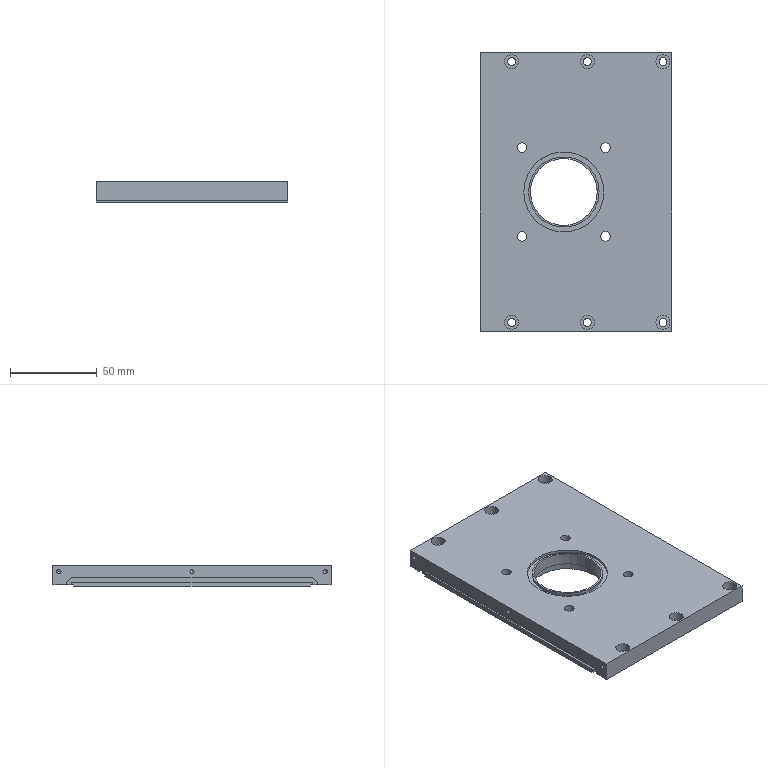NC program | NX | posted with a generic post | part box 110 x 160 x 12 mm
Lines 31 to 887 of 4419:
(ZLEVEL_PROFILE_COPY , TOOL : D3)
N54 T17 M6
N56 G54
N58 G17 G0 G90 X-46.066 Y1.694 B0. C0. S6260 M3
N60 G43 Z30. H17
N62 Z1.
N64 G94 G1 X-46.26 Y1.5 Z0.986 F1100.
N66 X-46.397 Y1.154 Z0.966
N68 X-46.384 Y0.783 Z0.947
N70 X-46.223 Y0.448 Z0.927
N72 X-46.03 Y0.261 Z0.913
N74 X-45.842 Y0.157 Z0.902
N76 X-45.635 Y0.1 Z0.891
N78 X-44.365 Z0.824
N80 X-44.064 Y0.201 Z0.807
N82 X-43.816 Y0.4 Z0.791
N84 X-43.651 Y0.672 Z0.774
N86 X-43.592 Y0.934 Z0.76
N88 X-43.631 Y1.27 Z0.742
N90 X-43.79 Y1.569 Z0.725
N92 X-44.046 Y1.789 Z0.707
N94 X-44.365 Y1.9 Z0.689
N96 X-45.635 Z0.623
N98 X-45.753 Y1.874 Z0.616
N100 X-45.997 Y1.762 Z0.602
N102 X-46.26 Y1.5 Z0.583
N104 X-46.397 Y1.154 Z0.563
N106 X-46.384 Y0.783 Z0.544
N108 X-46.223 Y0.448 Z0.524
N110 X-46.03 Y0.261 Z0.51
N112 X-45.842 Y0.157 Z0.499
N114 X-45.635 Y0.1 Z0.488
N116 X-44.365 Z0.421
N118 X-44.064 Y0.201 Z0.404
N120 X-43.816 Y0.4 Z0.388
N122 X-43.651 Y0.672 Z0.371
N124 X-43.592 Y0.934 Z0.357
N126 X-43.631 Y1.27 Z0.339
N128 X-43.79 Y1.569 Z0.322
N130 X-44.046 Y1.789 Z0.304
N132 X-44.365 Y1.9 Z0.286
N134 X-45.635 Z0.22
N136 X-45.753 Y1.874 Z0.213
N138 X-45.997 Y1.762 Z0.199
N140 X-46.26 Y1.5 Z0.18
N142 X-46.397 Y1.154 Z0.16
N144 X-46.384 Y0.783 Z0.141
N146 X-46.223 Y0.448 Z0.121
N148 X-46.03 Y0.261 Z0.107
N150 X-45.842 Y0.157 Z0.096
N152 X-45.635 Y0.1 Z0.085
N154 X-44.365 Z0.018
N156 X-44.064 Y0.201 Z0.002
N158 X-43.816 Y0.4 Z-0.015
N160 X-43.651 Y0.672 Z-0.032
N162 X-43.592 Y0.934 Z-0.046
N164 X-43.631 Y1.27 Z-0.064
N166 X-43.79 Y1.569 Z-0.081
N168 X-44.046 Y1.789 Z-0.099
N170 X-44.365 Y1.9 Z-0.117
N172 X-45. Z-0.15
N174 X-45.5
N176 G3 X-46.4 Y1. R0.9
N178 X-45.5 Y0.1 R0.9
N180 G1 X-44.5
N182 G3 X-43.6 Y1. R0.9
N184 X-44.5 Y1.9 R0.9
N186 G1 X-45.
N188 X-45.374 Z-0.16
N190 X-45.499 Y1.894 Z-0.163
N192 X-45.676 Y1.874 Z-0.168
N194 X-45.743 Y1.857 Z-0.17
N196 X-45.891 Y1.801 Z-0.174
N198 X-45.969 Y1.759 Z-0.176
N200 X-46.049 Y1.703 Z-0.179
N202 X-46.087 Y1.673 Z-0.18
N204 X-46.111 Y1.649 Z-0.181
N206 X-46.159 Y1.601 Z-0.183
N208 X-46.247 Y1.487 Z-0.186
N210 X-46.297 Y1.397 Z-0.189
N212 X-46.354 Y1.254 Z-0.193
N214 X-46.379 Y1.164 Z-0.196
N216 X-46.392 Y1.035 Z-0.199
N218 X-46.387 Y0.918 Z-0.202
N220 X-46.36 Y0.769 Z-0.206
N222 X-46.332 Y0.677 Z-0.209
N224 X-46.295 Y0.596 Z-0.211
N226 X-46.275 Y0.555 Z-0.212
N228 X-46.254 Y0.524 Z-0.213
N230 X-46.211 Y0.463 Z-0.215
N232 X-46.11 Y0.351 Z-0.219
N234 X-46.037 Y0.289 Z-0.222
N236 X-45.908 Y0.207 Z-0.226
N238 X-45.822 Y0.167 Z-0.228
N240 X-45.717 Y0.136 Z-0.231
N242 X-45.581 Y0.113 Z-0.235
N244 X-45.457 Y0.102 Z-0.238
N246 X-45.333 Y0.1 Z-0.241
N248 X-44.584 Z-0.261
N250 X-44.4 Y0.114 Z-0.266
N252 X-44.336 Y0.121 Z-0.267
N254 X-44.251 Y0.144 Z-0.27
N256 X-44.208 Y0.156 Z-0.271
N258 X-44.172 Y0.17 Z-0.272
N260 X-44.103 Y0.202 Z-0.274
N262 X-43.967 Y0.286 Z-0.278
N264 X-43.899 Y0.341 Z-0.28
N266 X-43.8 Y0.447 Z-0.284
N268 X-43.742 Y0.53 Z-0.287
N270 X-43.68 Y0.65 Z-0.291
N272 X-43.643 Y0.756 Z-0.293
N274 X-43.617 Y0.877 Z-0.297
N276 X-43.6 Y1. Z-0.3
N278 G3 X-44.5 Y1.9 R0.9
N280 G1 X-45.
N282 X-45.374 Z-0.31
N284 X-45.499 Y1.894 Z-0.313
N286 X-45.677 Y1.875 Z-0.318
N288 X-45.743 Y1.857 Z-0.32
N290 X-45.896 Y1.798 Z-0.324
N292 X-45.969 Y1.759 Z-0.326
N294 X-46.05 Y1.703 Z-0.329
N296 X-46.088 Y1.672 Z-0.33
N298 X-46.111 Y1.649 Z-0.331
N300 X-46.159 Y1.601 Z-0.333
N302 X-46.247 Y1.487 Z-0.336
N304 X-46.297 Y1.397 Z-0.339
N306 X-46.354 Y1.254 Z-0.343
N308 X-46.379 Y1.164 Z-0.346
N310 X-46.392 Y1.035 Z-0.349
N312 X-46.387 Y0.918 Z-0.352
N314 X-46.36 Y0.769 Z-0.356
N316 X-46.332 Y0.677 Z-0.359
N318 X-46.295 Y0.596 Z-0.361
N320 X-46.275 Y0.555 Z-0.362
N322 X-46.254 Y0.524 Z-0.363
N324 X-46.211 Y0.463 Z-0.365
N326 X-46.11 Y0.351 Z-0.369
N328 X-46.037 Y0.289 Z-0.372
N330 X-45.908 Y0.207 Z-0.376
N332 X-45.822 Y0.167 Z-0.378
N334 X-45.717 Y0.136 Z-0.381
N336 X-45.581 Y0.113 Z-0.385
N338 X-45.457 Y0.102 Z-0.388
N340 X-45.333 Y0.1 Z-0.391
N342 X-44.584 Z-0.411
N344 X-44.4 Y0.114 Z-0.416
N346 X-44.336 Y0.121 Z-0.417
N348 X-44.251 Y0.144 Z-0.42
N350 X-44.208 Y0.156 Z-0.421
N352 X-44.172 Y0.17 Z-0.422
N354 X-44.103 Y0.202 Z-0.424
N356 X-43.967 Y0.286 Z-0.428
N358 X-43.899 Y0.341 Z-0.43
N360 X-43.8 Y0.447 Z-0.434
N362 X-43.742 Y0.53 Z-0.437
N364 X-43.68 Y0.65 Z-0.441
N366 X-43.643 Y0.756 Z-0.443
N368 X-43.617 Y0.877 Z-0.447
N370 X-43.6 Y1. Z-0.45
N372 G3 X-44.5 Y1.9 R0.9
N374 G1 X-45.
N376 X-45.374 Z-0.46
N378 X-45.499 Y1.894 Z-0.463
N380 X-45.677 Y1.875 Z-0.468
N382 X-45.743 Y1.857 Z-0.47
N384 X-45.896 Y1.798 Z-0.474
N386 X-45.969 Y1.759 Z-0.476
N388 X-46.05 Y1.703 Z-0.479
N390 X-46.088 Y1.672 Z-0.48
N392 X-46.111 Y1.649 Z-0.481
N394 X-46.159 Y1.601 Z-0.483
N396 X-46.247 Y1.487 Z-0.486
N398 X-46.297 Y1.397 Z-0.489
N400 X-46.354 Y1.254 Z-0.493
N402 X-46.379 Y1.164 Z-0.496
N404 X-46.391 Y1.035 Z-0.499
N406 X-46.387 Y0.918 Z-0.502
N408 X-46.36 Y0.769 Z-0.506
N410 X-46.332 Y0.677 Z-0.509
N412 X-46.295 Y0.596 Z-0.511
N414 X-46.275 Y0.555 Z-0.512
N416 X-46.254 Y0.524 Z-0.513
N418 X-46.211 Y0.463 Z-0.515
N420 X-46.11 Y0.351 Z-0.519
N422 X-46.036 Y0.289 Z-0.522
N424 X-45.908 Y0.207 Z-0.526
N426 X-45.822 Y0.167 Z-0.528
N428 X-45.717 Y0.136 Z-0.531
N430 X-45.581 Y0.113 Z-0.535
N432 X-45.457 Y0.102 Z-0.538
N434 X-45.333 Y0.1 Z-0.541
N436 X-44.584 Z-0.561
N438 X-44.4 Y0.114 Z-0.566
N440 X-44.336 Y0.121 Z-0.567
N442 X-44.251 Y0.144 Z-0.57
N444 X-44.208 Y0.156 Z-0.571
N446 X-44.172 Y0.17 Z-0.572
N448 X-44.103 Y0.202 Z-0.574
N450 X-43.967 Y0.286 Z-0.578
N452 X-43.899 Y0.341 Z-0.58
N454 X-43.8 Y0.447 Z-0.584
N456 X-43.742 Y0.53 Z-0.587
N458 X-43.681 Y0.65 Z-0.59
N460 X-43.643 Y0.756 Z-0.593
N462 X-43.617 Y0.877 Z-0.597
N464 X-43.6 Y1. Z-0.6
N466 G3 X-44.5 Y1.9 R0.9
N468 G1 X-45.
N470 X-45.374 Z-0.61
N472 X-45.499 Y1.894 Z-0.613
N474 X-45.677 Y1.875 Z-0.618
N476 X-45.743 Y1.857 Z-0.62
N478 X-45.896 Y1.798 Z-0.624
N480 X-45.969 Y1.758 Z-0.626
N482 X-46.049 Y1.703 Z-0.629
N484 X-46.088 Y1.672 Z-0.63
N486 X-46.111 Y1.649 Z-0.631
N488 X-46.159 Y1.601 Z-0.633
N490 X-46.246 Y1.487 Z-0.636
N492 X-46.297 Y1.397 Z-0.639
N494 X-46.354 Y1.254 Z-0.643
N496 X-46.379 Y1.164 Z-0.646
N498 X-46.391 Y1.035 Z-0.649
N500 X-46.387 Y0.918 Z-0.652
N502 X-46.36 Y0.769 Z-0.656
N504 X-46.332 Y0.677 Z-0.659
N506 X-46.295 Y0.596 Z-0.661
N508 X-46.275 Y0.556 Z-0.662
N510 X-46.254 Y0.524 Z-0.663
N512 X-46.211 Y0.463 Z-0.665
N514 X-46.11 Y0.351 Z-0.669
N516 X-46.036 Y0.289 Z-0.672
N518 X-45.908 Y0.208 Z-0.676
N520 X-45.822 Y0.167 Z-0.678
N522 X-45.717 Y0.136 Z-0.681
N524 X-45.581 Y0.113 Z-0.685
N526 X-45.457 Y0.102 Z-0.688
N528 X-45.333 Y0.1 Z-0.691
N530 X-44.584 Z-0.711
N532 X-44.4 Y0.114 Z-0.716
N534 X-44.336 Y0.121 Z-0.717
N536 X-44.251 Y0.144 Z-0.72
N538 X-44.208 Y0.156 Z-0.721
N540 X-44.172 Y0.17 Z-0.722
N542 X-44.103 Y0.202 Z-0.724
N544 X-43.967 Y0.286 Z-0.728
N546 X-43.9 Y0.341 Z-0.73
N548 X-43.8 Y0.447 Z-0.734
N550 X-43.742 Y0.53 Z-0.737
N552 X-43.681 Y0.65 Z-0.74
N554 X-43.643 Y0.756 Z-0.743
N556 X-43.617 Y0.877 Z-0.747
N558 X-43.6 Y1. Z-0.75
N560 G3 X-44.5 Y1.9 R0.9
N562 G1 X-45.
N564 X-45.374 Z-0.76
N566 X-45.499 Y1.894 Z-0.763
N568 X-45.677 Y1.875 Z-0.768
N570 X-45.743 Y1.857 Z-0.77
N572 X-45.896 Y1.798 Z-0.774
N574 X-45.969 Y1.758 Z-0.776
N576 X-46.049 Y1.703 Z-0.779
N578 X-46.087 Y1.672 Z-0.78
N580 X-46.111 Y1.649 Z-0.781
N582 X-46.159 Y1.601 Z-0.783
N584 X-46.246 Y1.487 Z-0.786
N586 X-46.297 Y1.397 Z-0.789
N588 X-46.354 Y1.254 Z-0.793
N590 X-46.379 Y1.164 Z-0.796
N592 X-46.391 Y1.035 Z-0.799
N594 X-46.387 Y0.918 Z-0.802
N596 X-46.36 Y0.769 Z-0.806
N598 X-46.332 Y0.677 Z-0.809
N600 X-46.295 Y0.596 Z-0.811
N602 X-46.275 Y0.556 Z-0.812
N604 X-46.254 Y0.525 Z-0.813
N606 X-46.211 Y0.463 Z-0.815
N608 X-46.11 Y0.351 Z-0.819
N610 X-46.036 Y0.289 Z-0.822
N612 X-45.908 Y0.208 Z-0.826
N614 X-45.822 Y0.167 Z-0.828
N616 X-45.717 Y0.136 Z-0.831
N618 X-45.581 Y0.113 Z-0.835
N620 X-45.457 Y0.102 Z-0.838
N622 X-45.333 Y0.1 Z-0.841
N624 X-44.584 Z-0.861
N626 X-44.4 Y0.114 Z-0.866
N628 X-44.336 Y0.121 Z-0.867
N630 X-44.251 Y0.144 Z-0.87
N632 X-44.208 Y0.156 Z-0.871
N634 X-44.172 Y0.17 Z-0.872
N636 X-44.103 Y0.202 Z-0.874
N638 X-43.968 Y0.286 Z-0.878
N640 X-43.9 Y0.341 Z-0.88
N642 X-43.8 Y0.447 Z-0.884
N644 X-43.742 Y0.53 Z-0.887
N646 X-43.681 Y0.65 Z-0.89
N648 X-43.643 Y0.756 Z-0.893
N650 X-43.617 Y0.877 Z-0.897
N652 X-43.6 Y1. Z-0.9
N654 G3 X-44.5 Y1.9 R0.9
N656 G1 X-45.
N658 X-45.374 Z-0.91
N660 X-45.499 Y1.894 Z-0.913
N662 X-45.677 Y1.875 Z-0.918
N664 X-45.743 Y1.857 Z-0.92
N666 X-45.896 Y1.798 Z-0.924
N668 X-45.969 Y1.758 Z-0.926
N670 X-46.049 Y1.703 Z-0.929
N672 X-46.087 Y1.672 Z-0.93
N674 X-46.111 Y1.649 Z-0.931
N676 X-46.159 Y1.601 Z-0.933
N678 X-46.246 Y1.487 Z-0.936
N680 X-46.297 Y1.397 Z-0.939
N682 X-46.354 Y1.254 Z-0.943
N684 X-46.379 Y1.164 Z-0.946
N686 X-46.391 Y1.035 Z-0.949
N688 X-46.387 Y0.918 Z-0.952
N690 X-46.36 Y0.769 Z-0.956
N692 X-46.332 Y0.677 Z-0.959
N694 X-46.295 Y0.596 Z-0.961
N696 X-46.275 Y0.556 Z-0.962
N698 X-46.254 Y0.525 Z-0.963
N700 X-46.211 Y0.463 Z-0.965
N702 X-46.11 Y0.351 Z-0.969
N704 X-46.036 Y0.289 Z-0.972
N706 X-45.908 Y0.208 Z-0.976
N708 X-45.822 Y0.167 Z-0.978
N710 X-45.717 Y0.136 Z-0.981
N712 X-45.581 Y0.113 Z-0.985
N714 X-45.457 Y0.102 Z-0.988
N716 X-45.333 Y0.1 Z-0.991
N718 X-44.584 Z-1.011
N720 X-44.4 Y0.114 Z-1.016
N722 X-44.336 Y0.121 Z-1.017
N724 X-44.208 Y0.156 Z-1.021
N726 X-44.103 Y0.202 Z-1.024
N728 X-43.975 Y0.281 Z-1.028
N730 X-43.9 Y0.341 Z-1.03
N732 X-43.832 Y0.409 Z-1.033
N734 X-43.801 Y0.444 Z-1.034
N736 X-43.781 Y0.473 Z-1.035
N738 X-43.742 Y0.53 Z-1.037
N740 X-43.68 Y0.652 Z-1.041
N742 X-43.643 Y0.756 Z-1.043
N744 X-43.617 Y0.877 Z-1.047
N746 X-43.6 Y1. Z-1.05
N748 G3 X-44.5 Y1.9 R0.9
N750 G1 X-45.
N752 X-45.374 Z-1.06
N754 X-45.499 Y1.894 Z-1.063
N756 X-45.677 Y1.875 Z-1.068
N758 X-45.743 Y1.857 Z-1.07
N760 X-45.896 Y1.798 Z-1.074
N762 X-45.969 Y1.758 Z-1.076
N764 X-46.049 Y1.703 Z-1.079
N766 X-46.087 Y1.672 Z-1.08
N768 X-46.111 Y1.649 Z-1.081
N770 X-46.159 Y1.601 Z-1.083
N772 X-46.246 Y1.487 Z-1.086
N774 X-46.297 Y1.397 Z-1.089
N776 X-46.354 Y1.254 Z-1.093
N778 X-46.378 Y1.164 Z-1.096
N780 X-46.391 Y1.035 Z-1.099
N782 X-46.387 Y0.918 Z-1.102
N784 X-46.36 Y0.769 Z-1.106
N786 X-46.332 Y0.677 Z-1.109
N788 X-46.295 Y0.596 Z-1.111
N790 X-46.275 Y0.556 Z-1.112
N792 X-46.254 Y0.525 Z-1.113
N794 X-46.211 Y0.463 Z-1.115
N796 X-46.111 Y0.351 Z-1.119
N798 X-46.036 Y0.289 Z-1.122
N800 X-45.908 Y0.208 Z-1.126
N802 X-45.822 Y0.167 Z-1.128
N804 X-45.718 Y0.136 Z-1.131
N806 X-45.581 Y0.113 Z-1.135
N808 X-45.457 Y0.102 Z-1.138
N810 X-45.333 Y0.1 Z-1.141
N812 X-44.584 Z-1.161
N814 X-44.4 Y0.114 Z-1.166
N816 X-44.336 Y0.121 Z-1.167
N818 X-44.208 Y0.156 Z-1.171
N820 X-44.103 Y0.202 Z-1.174
N822 X-43.975 Y0.281 Z-1.178
N824 X-43.9 Y0.341 Z-1.18
N826 X-43.832 Y0.408 Z-1.183
N828 X-43.801 Y0.444 Z-1.184
N830 X-43.781 Y0.473 Z-1.185
N832 X-43.742 Y0.53 Z-1.187
N834 X-43.68 Y0.652 Z-1.191
N836 X-43.643 Y0.756 Z-1.193
N838 X-43.617 Y0.877 Z-1.197
N840 X-43.6 Y1. Z-1.2
N842 G3 X-44.5 Y1.9 R0.9
N844 G1 X-45.
N846 X-45.374 Z-1.21
N848 X-45.499 Y1.894 Z-1.213
N850 X-45.677 Y1.875 Z-1.218
N852 X-45.743 Y1.857 Z-1.22
N854 X-45.895 Y1.798 Z-1.224
N856 X-45.969 Y1.758 Z-1.226
N858 X-46.049 Y1.703 Z-1.229
N860 X-46.087 Y1.672 Z-1.23
N862 X-46.111 Y1.649 Z-1.231
N864 X-46.159 Y1.601 Z-1.233
N866 X-46.246 Y1.487 Z-1.236
N868 X-46.297 Y1.397 Z-1.239
N870 X-46.354 Y1.254 Z-1.243
N872 X-46.378 Y1.164 Z-1.246
N874 X-46.391 Y1.035 Z-1.249
N876 X-46.387 Y0.918 Z-1.252
N878 X-46.36 Y0.769 Z-1.256
N880 X-46.332 Y0.677 Z-1.259
N882 X-46.295 Y0.596 Z-1.261
N884 X-46.275 Y0.556 Z-1.262
N886 X-46.254 Y0.525 Z-1.263
N888 X-46.211 Y0.463 Z-1.265
N890 X-46.111 Y0.351 Z-1.269
N892 X-46.036 Y0.289 Z-1.272
N894 X-45.908 Y0.208 Z-1.276
N896 X-45.822 Y0.167 Z-1.278
N898 X-45.718 Y0.136 Z-1.281
N900 X-45.581 Y0.113 Z-1.285
N902 X-45.457 Y0.102 Z-1.288
N904 X-45.333 Y0.1 Z-1.291
N906 X-44.584 Z-1.311
N908 X-44.4 Y0.114 Z-1.316
N910 X-44.336 Y0.121 Z-1.317
N912 X-44.208 Y0.156 Z-1.321
N914 X-44.103 Y0.202 Z-1.324
N916 X-43.975 Y0.281 Z-1.328
N918 X-43.9 Y0.341 Z-1.33
N920 X-43.832 Y0.408 Z-1.333
N922 X-43.801 Y0.444 Z-1.334
N924 X-43.782 Y0.473 Z-1.335
N926 X-43.742 Y0.53 Z-1.337
N928 X-43.68 Y0.652 Z-1.341
N930 X-43.643 Y0.756 Z-1.343
N932 X-43.617 Y0.877 Z-1.347
N934 X-43.6 Y1. Z-1.35
N936 G3 X-44.5 Y1.9 R0.9
N938 G1 X-45.
N940 X-45.374 Z-1.36
N942 X-45.499 Y1.894 Z-1.363
N944 X-45.677 Y1.875 Z-1.368
N946 X-45.743 Y1.857 Z-1.37
N948 X-45.895 Y1.798 Z-1.374
N950 X-45.969 Y1.758 Z-1.376
N952 X-46.049 Y1.703 Z-1.379
N954 X-46.087 Y1.672 Z-1.38
N956 X-46.111 Y1.649 Z-1.381
N958 X-46.159 Y1.601 Z-1.383
N960 X-46.246 Y1.487 Z-1.386
N962 X-46.297 Y1.397 Z-1.389
N964 X-46.354 Y1.254 Z-1.393
N966 X-46.378 Y1.164 Z-1.396
N968 X-46.391 Y1.035 Z-1.399
N970 X-46.387 Y0.918 Z-1.402
N972 X-46.36 Y0.77 Z-1.406
N974 X-46.332 Y0.677 Z-1.409
N976 X-46.295 Y0.596 Z-1.411
N978 X-46.275 Y0.556 Z-1.412
N980 X-46.254 Y0.525 Z-1.413
N982 X-46.211 Y0.463 Z-1.415
N984 X-46.111 Y0.351 Z-1.419
N986 X-46.036 Y0.289 Z-1.422
N988 X-45.908 Y0.208 Z-1.426
N990 X-45.822 Y0.167 Z-1.428
N992 X-45.718 Y0.136 Z-1.431
N994 X-45.581 Y0.113 Z-1.435
N996 X-45.457 Y0.102 Z-1.438
N998 X-45.333 Y0.1 Z-1.441
N1000 X-44.584 Z-1.461
N1002 X-44.4 Y0.114 Z-1.466
N1004 X-44.336 Y0.121 Z-1.467
N1006 X-44.208 Y0.156 Z-1.471
N1008 X-44.103 Y0.202 Z-1.474
N1010 X-43.975 Y0.281 Z-1.478
N1012 X-43.9 Y0.341 Z-1.48
N1014 X-43.833 Y0.408 Z-1.483
N1016 X-43.801 Y0.444 Z-1.484
N1018 X-43.782 Y0.473 Z-1.485
N1020 X-43.742 Y0.53 Z-1.487
N1022 X-43.68 Y0.652 Z-1.491
N1024 X-43.643 Y0.756 Z-1.493
N1026 X-43.617 Y0.877 Z-1.497
N1028 X-43.6 Y1. Z-1.5
N1030 G3 X-44.5 Y1.9 R0.9
N1032 G1 X-45.
N1034 X-45.374 Z-1.51
N1036 X-45.499 Y1.894 Z-1.513
N1038 X-45.677 Y1.875 Z-1.518
N1040 X-45.743 Y1.857 Z-1.52
N1042 X-45.895 Y1.798 Z-1.524
N1044 X-45.969 Y1.758 Z-1.526
N1046 X-46.049 Y1.703 Z-1.529
N1048 X-46.087 Y1.673 Z-1.53
N1050 X-46.111 Y1.649 Z-1.531
N1052 X-46.159 Y1.601 Z-1.533
N1054 X-46.246 Y1.488 Z-1.536
N1056 X-46.297 Y1.397 Z-1.539
N1058 X-46.354 Y1.254 Z-1.543
N1060 X-46.378 Y1.164 Z-1.546
N1062 X-46.391 Y1.035 Z-1.549
N1064 X-46.387 Y0.918 Z-1.552
N1066 X-46.36 Y0.77 Z-1.556
N1068 X-46.332 Y0.677 Z-1.559
N1070 X-46.295 Y0.596 Z-1.561
N1072 X-46.275 Y0.556 Z-1.562
N1074 X-46.254 Y0.525 Z-1.563
N1076 X-46.211 Y0.463 Z-1.565
N1078 X-46.111 Y0.351 Z-1.569
N1080 X-46.036 Y0.289 Z-1.572
N1082 X-45.908 Y0.208 Z-1.576
N1084 X-45.822 Y0.167 Z-1.578
N1086 X-45.718 Y0.136 Z-1.581
N1088 X-45.581 Y0.113 Z-1.585
N1090 X-45.457 Y0.102 Z-1.588
N1092 X-45.333 Y0.1 Z-1.591
N1094 X-44.584 Z-1.611
N1096 X-44.401 Y0.114 Z-1.616
N1098 X-44.336 Y0.121 Z-1.617
N1100 X-44.208 Y0.156 Z-1.621
N1102 X-44.103 Y0.202 Z-1.624
N1104 X-43.975 Y0.281 Z-1.628
N1106 X-43.9 Y0.341 Z-1.63
N1108 X-43.801 Y0.444 Z-1.634
N1110 X-43.742 Y0.53 Z-1.637
N1112 X-43.68 Y0.651 Z-1.641
N1114 X-43.643 Y0.756 Z-1.643
N1116 X-43.616 Y0.877 Z-1.647
N1118 X-43.6 Y1. Z-1.65
N1120 G3 X-44.5 Y1.9 R0.9
N1122 G1 X-45.
N1124 X-45.374 Z-1.66
N1126 X-45.499 Y1.894 Z-1.663
N1128 X-45.677 Y1.875 Z-1.668
N1130 X-45.743 Y1.857 Z-1.67
N1132 X-45.895 Y1.798 Z-1.674
N1134 X-45.969 Y1.758 Z-1.676
N1136 X-46.049 Y1.703 Z-1.679
N1138 X-46.087 Y1.673 Z-1.68
N1140 X-46.111 Y1.649 Z-1.681
N1142 X-46.159 Y1.601 Z-1.683
N1144 X-46.246 Y1.488 Z-1.686
N1146 X-46.297 Y1.397 Z-1.689
N1148 X-46.354 Y1.254 Z-1.693
N1150 X-46.378 Y1.164 Z-1.696
N1152 X-46.391 Y1.035 Z-1.699
N1154 X-46.387 Y0.918 Z-1.702
N1156 X-46.361 Y0.769 Z-1.706
N1158 X-46.332 Y0.677 Z-1.709
N1160 X-46.275 Y0.553 Z-1.712
N1162 X-46.211 Y0.463 Z-1.715
N1164 X-46.109 Y0.35 Z-1.719
N1166 X-46.036 Y0.289 Z-1.722
N1168 X-45.908 Y0.208 Z-1.726
N1170 X-45.822 Y0.167 Z-1.728
N1172 X-45.718 Y0.136 Z-1.731
N1174 X-45.581 Y0.113 Z-1.735
N1176 X-45.457 Y0.102 Z-1.738
N1178 X-45.333 Y0.1 Z-1.741
N1180 X-44.584 Z-1.761
N1182 X-44.401 Y0.114 Z-1.766
N1184 X-44.336 Y0.121 Z-1.767
N1186 X-44.208 Y0.156 Z-1.771
N1188 X-44.103 Y0.202 Z-1.774
N1190 X-43.975 Y0.281 Z-1.778
N1192 X-43.9 Y0.341 Z-1.78
N1194 X-43.802 Y0.444 Z-1.784
N1196 X-43.742 Y0.53 Z-1.787
N1198 X-43.68 Y0.651 Z-1.791
N1200 X-43.643 Y0.756 Z-1.793
N1202 X-43.616 Y0.877 Z-1.797
N1204 X-43.6 Y1. Z-1.8
N1206 G3 X-44.5 Y1.9 R0.9
N1208 G1 X-45.
N1210 X-45.374 Z-1.81
N1212 X-45.499 Y1.894 Z-1.813
N1214 X-45.677 Y1.875 Z-1.818
N1216 X-45.743 Y1.857 Z-1.82
N1218 X-45.895 Y1.798 Z-1.824
N1220 X-45.969 Y1.758 Z-1.826
N1222 X-46.087 Y1.673 Z-1.83
N1224 X-46.159 Y1.601 Z-1.833
N1226 X-46.246 Y1.488 Z-1.836
N1228 X-46.297 Y1.397 Z-1.839
N1230 X-46.354 Y1.254 Z-1.843
N1232 X-46.378 Y1.164 Z-1.846
N1234 X-46.391 Y1.035 Z-1.849
N1236 X-46.387 Y0.918 Z-1.852
N1238 X-46.361 Y0.77 Z-1.856
N1240 X-46.332 Y0.677 Z-1.859
N1242 X-46.275 Y0.553 Z-1.862
N1244 X-46.211 Y0.463 Z-1.865
N1246 X-46.109 Y0.35 Z-1.869
N1248 X-46.036 Y0.289 Z-1.872
N1250 X-45.908 Y0.208 Z-1.876
N1252 X-45.822 Y0.167 Z-1.878
N1254 X-45.718 Y0.137 Z-1.881
N1256 X-45.581 Y0.113 Z-1.885
N1258 X-45.457 Y0.102 Z-1.888
N1260 X-45.333 Y0.1 Z-1.891
N1262 X-44.584 Z-1.911
N1264 X-44.401 Y0.114 Z-1.916
N1266 X-44.336 Y0.121 Z-1.917
N1268 X-44.208 Y0.156 Z-1.921
N1270 X-44.103 Y0.202 Z-1.924
N1272 X-43.975 Y0.281 Z-1.928
N1274 X-43.9 Y0.341 Z-1.93
N1276 X-43.802 Y0.444 Z-1.934
N1278 X-43.742 Y0.53 Z-1.937
N1280 X-43.68 Y0.651 Z-1.941
N1282 X-43.643 Y0.756 Z-1.943
N1284 X-43.616 Y0.877 Z-1.947
N1286 X-43.6 Y1. Z-1.95
N1288 G3 X-44.5 Y1.9 R0.9
N1290 G1 X-45.
N1292 X-45.374 Z-1.96
N1294 X-45.499 Y1.894 Z-1.963
N1296 X-45.677 Y1.875 Z-1.968
N1298 X-45.743 Y1.857 Z-1.97
N1300 X-45.895 Y1.798 Z-1.974
N1302 X-45.969 Y1.758 Z-1.976
N1304 X-46.087 Y1.673 Z-1.98
N1306 X-46.159 Y1.601 Z-1.983
N1308 X-46.246 Y1.488 Z-1.986
N1310 X-46.297 Y1.397 Z-1.989
N1312 X-46.354 Y1.254 Z-1.993
N1314 X-46.378 Y1.164 Z-1.996
N1316 X-46.391 Y1.035 Z-1.999
N1318 X-46.387 Y0.918 Z-2.002
N1320 X-46.361 Y0.77 Z-2.006
N1322 X-46.332 Y0.677 Z-2.009
N1324 X-46.275 Y0.553 Z-2.012
N1326 X-46.211 Y0.463 Z-2.015
N1328 X-46.109 Y0.35 Z-2.019
N1330 X-46.036 Y0.289 Z-2.022
N1332 X-45.908 Y0.208 Z-2.026
N1334 X-45.822 Y0.167 Z-2.028
N1336 X-45.718 Y0.137 Z-2.031
N1338 X-45.581 Y0.113 Z-2.035
N1340 X-45.457 Y0.102 Z-2.038
N1342 X-45.333 Y0.1 Z-2.041
N1344 X-44.584 Z-2.061
N1346 X-44.401 Y0.114 Z-2.066
N1348 X-44.336 Y0.121 Z-2.067
N1350 X-44.208 Y0.156 Z-2.071
N1352 X-44.103 Y0.202 Z-2.074
N1354 X-43.975 Y0.281 Z-2.078
N1356 X-43.9 Y0.341 Z-2.08
N1358 X-43.802 Y0.444 Z-2.084
N1360 X-43.742 Y0.53 Z-2.087
N1362 X-43.68 Y0.651 Z-2.091
N1364 X-43.643 Y0.756 Z-2.093
N1366 X-43.616 Y0.877 Z-2.097
N1368 X-43.6 Y1. Z-2.1
N1370 G3 X-44.5 Y1.9 R0.9
N1372 G1 X-45.
N1374 X-45.374 Z-2.11
N1376 X-45.499 Y1.894 Z-2.113
N1378 X-45.677 Y1.875 Z-2.118
N1380 X-45.743 Y1.857 Z-2.12
N1382 X-45.895 Y1.798 Z-2.124
N1384 X-45.969 Y1.758 Z-2.126
N1386 X-46.087 Y1.673 Z-2.13
N1388 X-46.159 Y1.601 Z-2.133
N1390 X-46.245 Y1.488 Z-2.136
N1392 X-46.297 Y1.397 Z-2.139
N1394 X-46.354 Y1.255 Z-2.143
N1396 X-46.378 Y1.164 Z-2.146
N1398 X-46.391 Y1.035 Z-2.149
N1400 X-46.387 Y0.918 Z-2.152
N1402 X-46.361 Y0.77 Z-2.156
N1404 X-46.332 Y0.677 Z-2.159
N1406 X-46.275 Y0.553 Z-2.162
N1408 X-46.211 Y0.463 Z-2.165
N1410 X-46.109 Y0.35 Z-2.169
N1412 X-46.036 Y0.289 Z-2.172
N1414 X-45.908 Y0.208 Z-2.176
N1416 X-45.822 Y0.167 Z-2.178
N1418 X-45.718 Y0.137 Z-2.181
N1420 X-45.581 Y0.113 Z-2.185
N1422 X-45.457 Y0.102 Z-2.188
N1424 X-45.333 Y0.1 Z-2.191
N1426 X-44.584 Z-2.211
N1428 X-44.401 Y0.115 Z-2.216
N1430 X-44.336 Y0.122 Z-2.217
N1432 X-44.209 Y0.156 Z-2.221
N1434 X-44.104 Y0.203 Z-2.224
N1436 X-43.976 Y0.281 Z-2.228
N1438 X-43.9 Y0.341 Z-2.23
N1440 X-43.802 Y0.444 Z-2.234
N1442 X-43.742 Y0.53 Z-2.237
N1444 X-43.68 Y0.651 Z-2.241
N1446 X-43.643 Y0.756 Z-2.243
N1448 X-43.616 Y0.877 Z-2.247
N1450 X-43.6 Y1. Z-2.25
N1452 G3 X-44.5 Y1.9 R0.9
N1454 G1 X-45.
N1456 X-45.374 Z-2.26
N1458 X-45.499 Y1.894 Z-2.263
N1460 X-45.678 Y1.875 Z-2.268
N1462 X-45.743 Y1.857 Z-2.27
N1464 X-45.895 Y1.798 Z-2.274
N1466 X-45.969 Y1.758 Z-2.276
N1468 X-46.087 Y1.673 Z-2.28
N1470 X-46.159 Y1.601 Z-2.283
N1472 X-46.245 Y1.488 Z-2.286
N1474 X-46.297 Y1.397 Z-2.289
N1476 X-46.353 Y1.255 Z-2.293
N1478 X-46.378 Y1.164 Z-2.296
N1480 X-46.391 Y1.036 Z-2.299
N1482 X-46.387 Y0.918 Z-2.302
N1484 X-46.361 Y0.77 Z-2.306
N1486 X-46.332 Y0.677 Z-2.309
N1488 X-46.275 Y0.554 Z-2.312
N1490 X-46.211 Y0.463 Z-2.315
N1492 X-46.109 Y0.35 Z-2.319
N1494 X-46.036 Y0.289 Z-2.322
N1496 X-45.908 Y0.208 Z-2.326
N1498 X-45.822 Y0.167 Z-2.328
N1500 X-45.718 Y0.137 Z-2.331
N1502 X-45.581 Y0.113 Z-2.335
N1504 X-45.457 Y0.102 Z-2.338
N1506 X-45.333 Y0.1 Z-2.341
N1508 X-44.584 Z-2.361
N1510 X-44.401 Y0.115 Z-2.366
N1512 X-44.336 Y0.122 Z-2.367
N1514 X-44.209 Y0.156 Z-2.371
N1516 X-44.104 Y0.203 Z-2.374
N1518 X-43.976 Y0.281 Z-2.378
N1520 X-43.9 Y0.341 Z-2.38
N1522 X-43.802 Y0.444 Z-2.384
N1524 X-43.742 Y0.53 Z-2.387
N1526 X-43.681 Y0.651 Z-2.391
N1528 X-43.643 Y0.756 Z-2.393
N1530 X-43.616 Y0.877 Z-2.397
N1532 X-43.6 Y1. Z-2.4
N1534 G3 X-44.5 Y1.9 R0.9
N1536 G1 X-45.
N1538 X-45.374 Z-2.41
N1540 X-45.499 Y1.894 Z-2.413
N1542 X-45.678 Y1.875 Z-2.418
N1544 X-45.743 Y1.857 Z-2.42
N1546 X-45.895 Y1.798 Z-2.424
N1548 X-45.969 Y1.758 Z-2.426
N1550 X-46.086 Y1.673 Z-2.43
N1552 X-46.159 Y1.601 Z-2.433
N1554 X-46.245 Y1.488 Z-2.436
N1556 X-46.297 Y1.397 Z-2.439
N1558 X-46.353 Y1.255 Z-2.443
N1560 X-46.378 Y1.164 Z-2.446
N1562 X-46.391 Y1.036 Z-2.449
N1564 X-46.387 Y0.918 Z-2.452
N1566 X-46.361 Y0.77 Z-2.456
N1568 X-46.332 Y0.677 Z-2.459
N1570 X-46.275 Y0.554 Z-2.462
N1572 X-46.211 Y0.463 Z-2.465
N1574 X-46.109 Y0.35 Z-2.469
N1576 X-46.036 Y0.289 Z-2.472
N1578 X-45.908 Y0.208 Z-2.476
N1580 X-45.822 Y0.168 Z-2.478
N1582 X-45.718 Y0.137 Z-2.481
N1584 X-45.581 Y0.113 Z-2.485
N1586 X-45.457 Y0.103 Z-2.488
N1588 X-45.333 Y0.1 Z-2.491
N1590 X-44.584 Z-2.511
N1592 X-44.401 Y0.115 Z-2.516
N1594 X-44.336 Y0.122 Z-2.517
N1596 X-44.209 Y0.156 Z-2.521
N1598 X-44.104 Y0.203 Z-2.524
N1600 X-43.976 Y0.281 Z-2.528
N1602 X-43.9 Y0.341 Z-2.53
N1604 X-43.802 Y0.444 Z-2.534
N1606 X-43.742 Y0.53 Z-2.537
N1608 X-43.681 Y0.651 Z-2.541
N1610 X-43.643 Y0.756 Z-2.543
N1612 X-43.616 Y0.877 Z-2.547
N1614 X-43.6 Y1. Z-2.55
N1616 G3 X-44.5 Y1.9 R0.9
N1618 G1 X-45.
N1620 X-45.374 Z-2.56
N1622 X-45.499 Y1.894 Z-2.563
N1624 X-45.678 Y1.875 Z-2.568
N1626 X-45.743 Y1.857 Z-2.57
N1628 X-45.895 Y1.798 Z-2.574
N1630 X-45.969 Y1.758 Z-2.576
N1632 X-46.086 Y1.673 Z-2.58
N1634 X-46.159 Y1.601 Z-2.583
N1636 X-46.245 Y1.488 Z-2.586
N1638 X-46.297 Y1.397 Z-2.589
N1640 X-46.353 Y1.255 Z-2.593
N1642 X-46.378 Y1.164 Z-2.596
N1644 X-46.391 Y1.036 Z-2.599
N1646 X-46.387 Y0.918 Z-2.602
N1648 X-46.361 Y0.77 Z-2.606
N1650 X-46.332 Y0.677 Z-2.609
N1652 X-46.275 Y0.554 Z-2.612
N1654 X-46.21 Y0.463 Z-2.615
N1656 X-46.109 Y0.351 Z-2.619
N1658 X-46.036 Y0.289 Z-2.622
N1660 X-45.908 Y0.208 Z-2.626
N1662 X-45.822 Y0.168 Z-2.628
N1664 X-45.718 Y0.137 Z-2.631
N1666 X-45.581 Y0.113 Z-2.635
N1668 X-45.457 Y0.103 Z-2.638
N1670 X-45.333 Y0.1 Z-2.641
N1672 X-44.584 Z-2.661
N1674 X-44.401 Y0.115 Z-2.666
N1676 X-44.336 Y0.122 Z-2.667
N1678 X-44.209 Y0.156 Z-2.671
N1680 X-44.104 Y0.203 Z-2.674
N1682 X-43.976 Y0.281 Z-2.678
N1684 X-43.9 Y0.341 Z-2.68
N1686 X-43.802 Y0.444 Z-2.684
N1688 X-43.742 Y0.53 Z-2.687
N1690 X-43.681 Y0.651 Z-2.691
N1692 X-43.643 Y0.756 Z-2.693
N1694 X-43.616 Y0.877 Z-2.697
N1696 X-43.6 Y1. Z-2.7
N1698 G3 X-44.5 Y1.9 R0.9
N1700 G1 X-45.
N1702 X-45.374 Z-2.71
N1704 X-45.499 Y1.894 Z-2.713
N1706 X-45.678 Y1.875 Z-2.718
N1708 X-45.743 Y1.857 Z-2.72
N1710 X-45.895 Y1.798 Z-2.724
N1712 X-45.969 Y1.758 Z-2.726
N1714 X-46.086 Y1.673 Z-2.73
N1716 X-46.159 Y1.601 Z-2.733
N1718 X-46.245 Y1.488 Z-2.736
N1720 X-46.297 Y1.397 Z-2.739
N1722 X-46.353 Y1.255 Z-2.743
N1724 X-46.378 Y1.164 Z-2.746
N1726 X-46.391 Y1.036 Z-2.749
N1728 X-46.387 Y0.918 Z-2.752
N1730 X-46.361 Y0.77 Z-2.756
N1732 X-46.332 Y0.677 Z-2.759
N1734 X-46.275 Y0.554 Z-2.762
N1736 X-46.21 Y0.463 Z-2.765
N1738 X-46.109 Y0.351 Z-2.769
N1740 X-46.036 Y0.289 Z-2.772
N1742 X-45.908 Y0.208 Z-2.776
N1744 X-45.822 Y0.168 Z-2.778
N1746 X-45.718 Y0.137 Z-2.781
N1748 X-45.581 Y0.113 Z-2.785
N1750 X-45.457 Y0.103 Z-2.788
N1752 X-45.333 Y0.1 Z-2.791
N1754 X-44.584 Z-2.811
N1756 X-44.401 Y0.115 Z-2.816
N1758 X-44.336 Y0.122 Z-2.817
N1760 X-44.209 Y0.156 Z-2.821